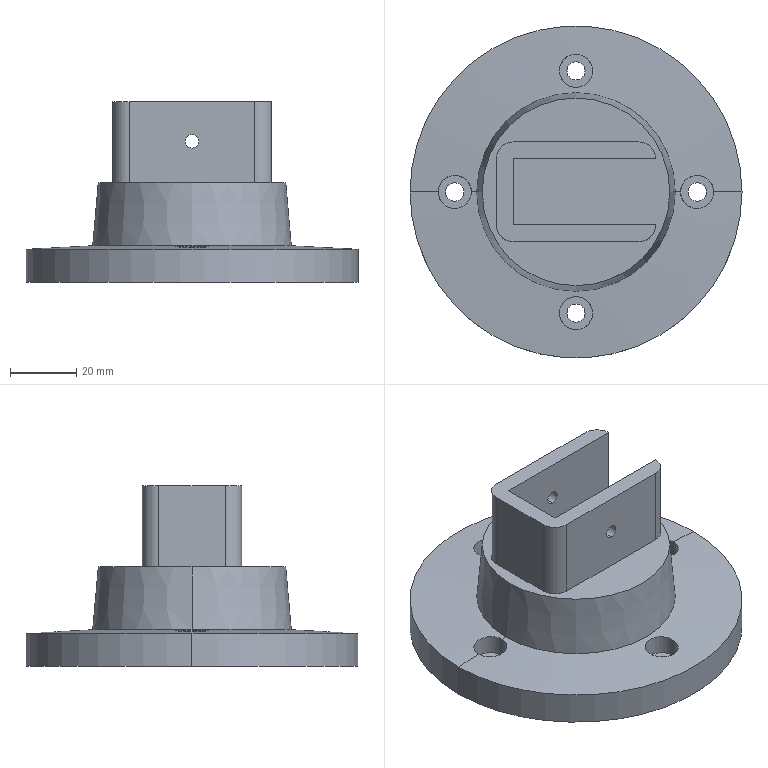Part | SolidWorks | features BaseBody 1 | 1 solid | 43 faces | box 100 x 100 x 54.5 mm | volume 145540 mm3 | cylinder 26 | plane 13 | cone 4 | commonest cylinder face diameters 10 x12 5.5 x8 4 x4 100 x2